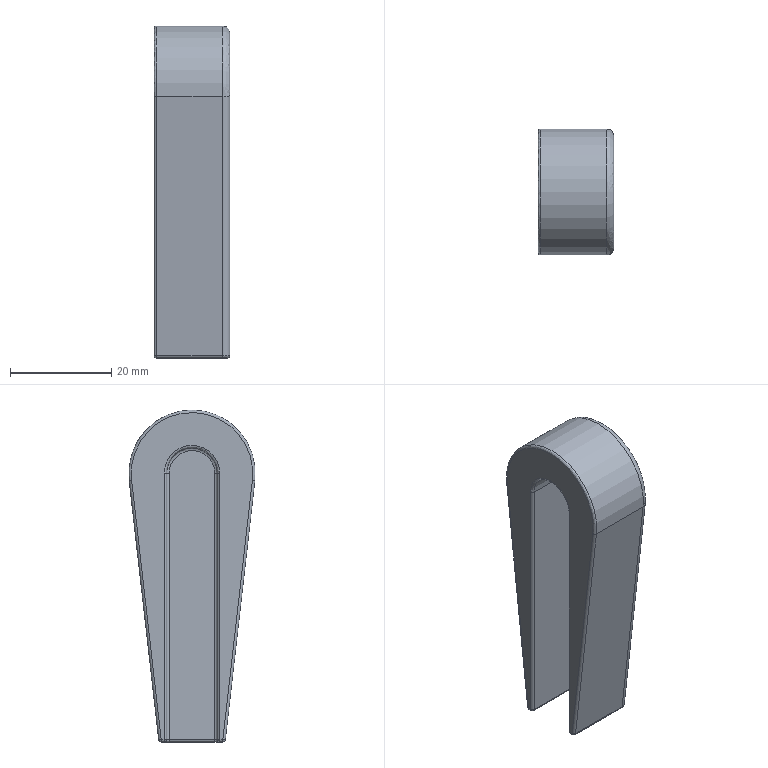Part | STEP file | ESG2 | 1 solid | 40 faces | box 15 x 25 x 65.581 mm | volume 10837 mm3 | cylinder 19 | spline 12 | plane 9 | commonest cylinder face diameters 1 x14 3 x2 10 x2 25 x1